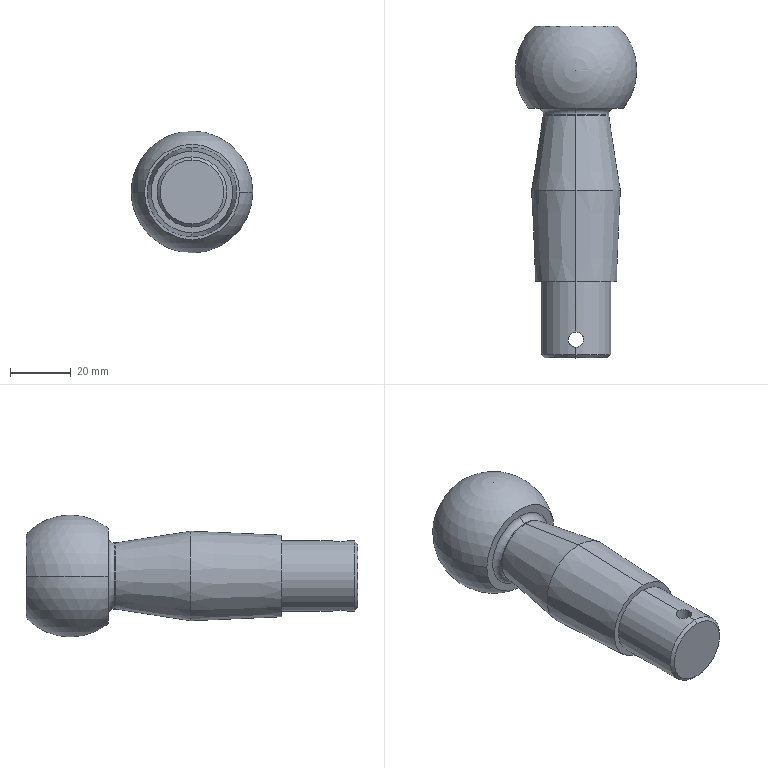Part | SolidWorks | features Chamfer 1, Fillet 1, ICE 1, Revolution 1 | 1 solid | 20 faces | box 40 x 109 x 40 mm | volume 70889 mm3 | cone 6 | torus 4 | cylinder 4 | plane 4 | sphere 2 | commonest cylinder face diameters 5 x2 23 x2
STEP:
#1=CARTESIAN_POINT('',(0.,-12.5,12.835));
#2=VERTEX_POINT('',#1);
#3=CARTESIAN_POINT('',(0.,-14.5,10.835));
#4=VERTEX_POINT('',#3);
#5=CARTESIAN_POINT('',(0.,-14.5,12.835));
#6=DIRECTION('',(-1.,0.,0.));
#7=DIRECTION('',(0.,0.,1.));
#8=AXIS2_PLACEMENT_3D('',#5,#6,#7);
#9=CIRCLE('',#8,2.);
#10=EDGE_CURVE('',#2,#4,#9,.T.);
#11=ORIENTED_EDGE('',*,*,#10,.T.);
#12=CARTESIAN_POINT('',(0.,-14.5,-10.835));
#13=VERTEX_POINT('',#12);
#14=CARTESIAN_POINT('',(0.,-14.5,0.));
#15=DIRECTION('',(0.,1.,0.));
#16=DIRECTION('',(0.,0.,1.));
#17=AXIS2_PLACEMENT_3D('',#14,#15,#16);
#18=CIRCLE('',#17,10.835);
#19=EDGE_CURVE('',#4,#13,#18,.T.);
#20=ORIENTED_EDGE('',*,*,#19,.T.);
#21=CARTESIAN_POINT('',(0.,-12.5,-12.835));
#22=VERTEX_POINT('',#21);
#23=CARTESIAN_POINT('',(0.,-14.5,-12.835));
#24=DIRECTION('',(1.,0.,0.));
#25=DIRECTION('',(0.,0.,-1.));
#26=AXIS2_PLACEMENT_3D('',#23,#24,#25);
#27=CIRCLE('',#26,2.);
#28=EDGE_CURVE('',#22,#13,#27,.T.);
#29=ORIENTED_EDGE('',*,*,#28,.F.);
#30=CARTESIAN_POINT('',(0.,-12.5,0.));
#31=DIRECTION('',(0.,1.,0.));
#32=DIRECTION('',(0.,0.,1.));
#33=AXIS2_PLACEMENT_3D('',#30,#31,#32);
#34=CIRCLE('',#33,12.835);
#35=EDGE_CURVE('',#2,#22,#34,.T.);
#36=ORIENTED_EDGE('',*,*,#35,.F.);
#37=EDGE_LOOP('',(#11,#20,#29,#36));
#38=FACE_OUTER_BOUND('',#37,.T.);
#39=CARTESIAN_POINT('',(0.,-14.5,0.));
#40=DIRECTION('',(0.,1.,0.));
#41=DIRECTION('',(0.,0.,1.));
#42=AXIS2_PLACEMENT_3D('',#39,#40,#41);
#43=TOROIDAL_SURFACE('',#42,12.835,2.);
#44=ADVANCED_FACE('',(#38),#43,.F.);
#45=ORIENTED_EDGE('',*,*,#28,.T.);
#46=CARTESIAN_POINT('',(0.,-14.5,0.));
#47=DIRECTION('',(0.,1.,0.));
#48=DIRECTION('',(0.,0.,1.));
#49=AXIS2_PLACEMENT_3D('',#46,#47,#48);
#50=CIRCLE('',#49,10.835);
#51=EDGE_CURVE('',#13,#4,#50,.T.);
#52=ORIENTED_EDGE('',*,*,#51,.T.);
#53=ORIENTED_EDGE('',*,*,#10,.F.);
#54=CARTESIAN_POINT('',(0.,-12.5,0.));
#55=DIRECTION('',(0.,1.,0.));
#56=DIRECTION('',(0.,0.,1.));
#57=AXIS2_PLACEMENT_3D('',#54,#55,#56);
#58=CIRCLE('',#57,12.835);
#59=EDGE_CURVE('',#22,#2,#58,.T.);
#60=ORIENTED_EDGE('',*,*,#59,.F.);
#61=EDGE_LOOP('',(#45,#52,#53,#60));
#62=FACE_OUTER_BOUND('',#61,.T.);
#63=CARTESIAN_POINT('',(0.,-14.5,0.));
#64=DIRECTION('',(0.,1.,0.));
#65=DIRECTION('',(0.,0.,1.));
#66=AXIS2_PLACEMENT_3D('',#63,#64,#65);
#67=TOROIDAL_SURFACE('',#66,12.835,2.);
#68=ADVANCED_FACE('',(#62),#67,.F.);
#69=CARTESIAN_POINT('',(-2.5,-88.5,-11.225));
#70=VERTEX_POINT('',#69);
#71=CARTESIAN_POINT('',(0.,-91.,-11.5));
#72=VERTEX_POINT('',#71);
#73=CARTESIAN_POINT('',(-2.5,-88.5,-11.225));
#74=CARTESIAN_POINT('',(-2.5,-88.827,-11.225));
#75=CARTESIAN_POINT('',(-2.434,-89.157,-11.24));
#76=CARTESIAN_POINT('',(-2.247,-89.608,-11.279));
#77=CARTESIAN_POINT('',(-2.169,-89.754,-11.294));
#78=CARTESIAN_POINT('',(-1.987,-90.026,-11.327));
#79=CARTESIAN_POINT('',(-1.884,-90.152,-11.345));
#80=CARTESIAN_POINT('',(-1.653,-90.382,-11.381));
#81=CARTESIAN_POINT('',(-1.525,-90.488,-11.399));
#82=CARTESIAN_POINT('',(-1.254,-90.669,-11.432));
#83=CARTESIAN_POINT('',(-1.111,-90.746,-11.447));
#84=CARTESIAN_POINT('',(-0.6555,-90.935,-11.485));
#85=CARTESIAN_POINT('',(-0.3301,-91.,-11.5));
#86=CARTESIAN_POINT('',(0.,-91.,-11.5));
#87=B_SPLINE_CURVE_WITH_KNOTS('',3,(#73,#74,#75,#76,#77,#78,#79,#80,#81,#82,#83,#84,#85,#86),.UNSPECIFIED.,.F.,.F.,(4,2,2,2,2,2,4),(0.00784,0.00882,0.009309,0.009799,0.01029,0.01078,0.01176),.UNSPECIFIED.);
#88=EDGE_CURVE('',#70,#72,#87,.T.);
#89=ORIENTED_EDGE('',*,*,#88,.F.);
#90=CARTESIAN_POINT('',(-2.5,-88.5,11.225));
#91=VERTEX_POINT('',#90);
#92=CARTESIAN_POINT('',(-2.5,-88.5,-20.));
#93=DIRECTION('',(0.,0.,1.));
#94=VECTOR('',#93,1000.);
#95=LINE('',#92,#94);
#96=EDGE_CURVE('',#70,#91,#95,.T.);
#97=ORIENTED_EDGE('',*,*,#96,.T.);
#98=CARTESIAN_POINT('',(0.,-91.,11.5));
#99=VERTEX_POINT('',#98);
#100=CARTESIAN_POINT('',(0.,-91.,11.5));
#101=CARTESIAN_POINT('',(-0.1658,-91.,11.5));
#102=CARTESIAN_POINT('',(-0.3286,-90.984,11.496));
#103=CARTESIAN_POINT('',(-0.6489,-90.92,11.483));
#104=CARTESIAN_POINT('',(-0.8081,-90.871,11.473));
#105=CARTESIAN_POINT('',(-1.111,-90.746,11.447));
#106=CARTESIAN_POINT('',(-1.254,-90.669,11.432));
#107=CARTESIAN_POINT('',(-1.526,-90.487,11.399));
#108=CARTESIAN_POINT('',(-1.654,-90.382,11.381));
#109=CARTESIAN_POINT('',(-1.998,-90.037,11.327));
#110=CARTESIAN_POINT('',(-2.184,-89.759,11.291));
#111=CARTESIAN_POINT('',(-2.372,-89.307,11.253));
#112=CARTESIAN_POINT('',(-2.42,-89.149,11.243));
#113=CARTESIAN_POINT('',(-2.484,-88.826,11.229));
#114=CARTESIAN_POINT('',(-2.5,-88.664,11.225));
#115=CARTESIAN_POINT('',(-2.5,-88.5,11.225));
#116=B_SPLINE_CURVE_WITH_KNOTS('',3,(#100,#101,#102,#103,#104,#105,#106,#107,#108,#109,#110,#111,#112,#113,#114,#115),.UNSPECIFIED.,.F.,.F.,(4,2,2,2,2,2,2,4),(0.,0.0004901,0.0009802,0.00147,0.00196,0.002941,0.003431,0.003921),.UNSPECIFIED.);
#117=EDGE_CURVE('',#99,#91,#116,.T.);
#118=ORIENTED_EDGE('',*,*,#117,.F.);
#119=CARTESIAN_POINT('',(2.5,-88.5,11.225));
#120=VERTEX_POINT('',#119);
#121=CARTESIAN_POINT('',(2.5,-88.5,11.225));
#122=CARTESIAN_POINT('',(2.5,-88.665,11.225));
#123=CARTESIAN_POINT('',(2.484,-88.828,11.229));
#124=CARTESIAN_POINT('',(2.42,-89.148,11.243));
#125=CARTESIAN_POINT('',(2.372,-89.307,11.253));
#126=CARTESIAN_POINT('',(2.246,-89.609,11.279));
#127=CARTESIAN_POINT('',(2.17,-89.753,11.294));
#128=CARTESIAN_POINT('',(1.988,-90.025,11.327));
#129=CARTESIAN_POINT('',(1.883,-90.152,11.345));
#130=CARTESIAN_POINT('',(1.539,-90.497,11.399));
#131=CARTESIAN_POINT('',(1.261,-90.683,11.435));
#132=CARTESIAN_POINT('',(0.8102,-90.871,11.472));
#133=CARTESIAN_POINT('',(0.6514,-90.919,11.483));
#134=CARTESIAN_POINT('',(0.329,-90.984,11.496));
#135=CARTESIAN_POINT('',(0.1656,-91.,11.5));
#136=CARTESIAN_POINT('',(0.,-91.,11.5));
#137=B_SPLINE_CURVE_WITH_KNOTS('',3,(#121,#122,#123,#124,#125,#126,#127,#128,#129,#130,#131,#132,#133,#134,#135,#136),.UNSPECIFIED.,.F.,.F.,(4,2,2,2,2,2,2,4),(0.01176,0.01225,0.01274,0.01323,0.01372,0.0147,0.01519,0.01568),.UNSPECIFIED.);
#138=EDGE_CURVE('',#120,#99,#137,.T.);
#139=ORIENTED_EDGE('',*,*,#138,.F.);
#140=CARTESIAN_POINT('',(2.5,-88.5,-11.225));
#141=VERTEX_POINT('',#140);
#142=CARTESIAN_POINT('',(2.5,-88.5,-20.));
#143=DIRECTION('',(0.,0.,1.));
#144=VECTOR('',#143,1000.);
#145=LINE('',#142,#144);
#146=EDGE_CURVE('',#141,#120,#145,.T.);
#147=ORIENTED_EDGE('',*,*,#146,.F.);
#148=CARTESIAN_POINT('',(0.,-91.,-11.5));
#149=CARTESIAN_POINT('',(0.1649,-91.,-11.5));
#150=CARTESIAN_POINT('',(0.3275,-90.984,-11.496));
#151=CARTESIAN_POINT('',(0.648,-90.92,-11.483));
#152=CARTESIAN_POINT('',(0.8074,-90.872,-11.473));
#153=CARTESIAN_POINT('',(1.109,-90.746,-11.447));
#154=CARTESIAN_POINT('',(1.253,-90.67,-11.432));
#155=CARTESIAN_POINT('',(1.525,-90.488,-11.399));
#156=CARTESIAN_POINT('',(1.652,-90.383,-11.381));
#157=CARTESIAN_POINT('',(1.997,-90.039,-11.328));
#158=CARTESIAN_POINT('',(2.183,-89.761,-11.292));
#159=CARTESIAN_POINT('',(2.371,-89.31,-11.253));
#160=CARTESIAN_POINT('',(2.419,-89.151,-11.243));
#161=CARTESIAN_POINT('',(2.484,-88.829,-11.229));
#162=CARTESIAN_POINT('',(2.5,-88.666,-11.225));
#163=CARTESIAN_POINT('',(2.5,-88.5,-11.225));
#164=B_SPLINE_CURVE_WITH_KNOTS('',3,(#148,#149,#150,#151,#152,#153,#154,#155,#156,#157,#158,#159,#160,#161,#162,#163),.UNSPECIFIED.,.F.,.F.,(4,2,2,2,2,2,2,4),(0.01176,0.01225,0.01274,0.01323,0.01372,0.0147,0.01519,0.01568),.UNSPECIFIED.);
#165=EDGE_CURVE('',#72,#141,#164,.T.);
#166=ORIENTED_EDGE('',*,*,#165,.F.);
#167=EDGE_LOOP('',(#89,#97,#118,#139,#147,#166));
#168=FACE_OUTER_BOUND('',#167,.T.);
#169=CARTESIAN_POINT('',(0.,-88.5,-20.));
#170=DIRECTION('',(0.,0.,1.));
#171=DIRECTION('',(1.,0.,0.));
#172=AXIS2_PLACEMENT_3D('',#169,#170,#171);
#173=CYLINDRICAL_SURFACE('',#172,2.5);
#174=ADVANCED_FACE('',(#168),#173,.F.);
#175=ORIENTED_EDGE('',*,*,#51,.F.);
#176=CARTESIAN_POINT('',(0.,-14.807,-10.859));
#177=VERTEX_POINT('',#176);
#178=CARTESIAN_POINT('',(0.,-14.5,-12.835));
#179=DIRECTION('',(1.,0.,0.));
#180=DIRECTION('',(0.,0.,-1.));
#181=AXIS2_PLACEMENT_3D('',#178,#179,#180);
#182=CIRCLE('',#181,2.);
#183=EDGE_CURVE('',#13,#177,#182,.T.);
#184=ORIENTED_EDGE('',*,*,#183,.T.);
#185=CARTESIAN_POINT('',(0.,-14.807,10.859));
#186=VERTEX_POINT('',#185);
#187=CARTESIAN_POINT('',(0.,-14.807,0.));
#188=DIRECTION('',(0.,-1.,0.));
#189=DIRECTION('',(0.,0.,-1.));
#190=AXIS2_PLACEMENT_3D('',#187,#188,#189);
#191=CIRCLE('',#190,10.859);
#192=EDGE_CURVE('',#186,#177,#191,.T.);
#193=ORIENTED_EDGE('',*,*,#192,.F.);
#194=CARTESIAN_POINT('',(0.,-14.5,12.835));
#195=DIRECTION('',(-1.,0.,0.));
#196=DIRECTION('',(0.,0.,1.));
#197=AXIS2_PLACEMENT_3D('',#194,#195,#196);
#198=CIRCLE('',#197,2.);
#199=EDGE_CURVE('',#4,#186,#198,.T.);
#200=ORIENTED_EDGE('',*,*,#199,.F.);
#201=EDGE_LOOP('',(#175,#184,#193,#200));
#202=FACE_OUTER_BOUND('',#201,.T.);
#203=CARTESIAN_POINT('',(0.,-14.5,0.));
#204=DIRECTION('',(0.,1.,0.));
#205=DIRECTION('',(0.,0.,1.));
#206=AXIS2_PLACEMENT_3D('',#203,#204,#205);
#207=TOROIDAL_SURFACE('',#206,12.835,2.);
#208=ADVANCED_FACE('',(#202),#207,.F.);
#209=CARTESIAN_POINT('',(0.,-94.5,-10.5));
#210=VERTEX_POINT('',#209);
#211=CARTESIAN_POINT('',(0.,-94.5,10.5));
#212=VERTEX_POINT('',#211);
#213=CARTESIAN_POINT('',(0.,-94.5,0.));
#214=DIRECTION('',(0.,-1.,0.));
#215=DIRECTION('',(0.,0.,1.));
#216=AXIS2_PLACEMENT_3D('',#213,#214,#215);
#217=CIRCLE('',#216,10.5);
#218=EDGE_CURVE('',#210,#212,#217,.T.);
#219=ORIENTED_EDGE('',*,*,#218,.F.);
#220=CARTESIAN_POINT('',(0.,-93.5,-11.5));
#221=VERTEX_POINT('',#220);
#222=CARTESIAN_POINT('',(0.,-93.5,-11.5));
#223=DIRECTION('',(0.,0.7071,-0.7071));
#224=VECTOR('',#223,1000.);
#225=LINE('',#222,#224);
#226=EDGE_CURVE('',#210,#221,#225,.T.);
#227=ORIENTED_EDGE('',*,*,#226,.T.);
#228=CARTESIAN_POINT('',(0.,-93.5,11.5));
#229=VERTEX_POINT('',#228);
#230=CARTESIAN_POINT('',(0.,-93.5,0.));
#231=DIRECTION('',(0.,1.,0.));
#232=DIRECTION('',(0.,0.,1.));
#233=AXIS2_PLACEMENT_3D('',#230,#231,#232);
#234=CIRCLE('',#233,11.5);
#235=EDGE_CURVE('',#229,#221,#234,.T.);
#236=ORIENTED_EDGE('',*,*,#235,.F.);
#237=CARTESIAN_POINT('',(0.,-93.5,11.5));
#238=DIRECTION('',(0.,0.7071,0.7071));
#239=VECTOR('',#238,1000.);
#240=LINE('',#237,#239);
#241=EDGE_CURVE('',#212,#229,#240,.T.);
#242=ORIENTED_EDGE('',*,*,#241,.F.);
#243=EDGE_LOOP('',(#219,#227,#236,#242));
#244=FACE_OUTER_BOUND('',#243,.T.);
#245=CARTESIAN_POINT('',(0.,-93.5,0.));
#246=DIRECTION('',(0.,1.,0.));
#247=DIRECTION('',(0.,0.,1.));
#248=AXIS2_PLACEMENT_3D('',#245,#246,#247);
#249=CONICAL_SURFACE('',#248,11.5,0.7854);
#250=ADVANCED_FACE('',(#244),#249,.T.);
#251=CARTESIAN_POINT('',(15.612,-12.5,0.));
#252=VERTEX_POINT('',#251);
#253=CARTESIAN_POINT('',(-15.612,-12.5,0.));
#254=VERTEX_POINT('',#253);
#255=CARTESIAN_POINT('',(0.,-12.5,0.));
#256=DIRECTION('',(0.,1.,0.));
#257=DIRECTION('',(0.,0.,1.));
#258=AXIS2_PLACEMENT_3D('',#255,#256,#257);
#259=CIRCLE('',#258,15.612);
#260=EDGE_CURVE('',#252,#254,#259,.T.);
#261=ORIENTED_EDGE('',*,*,#260,.T.);
#262=CARTESIAN_POINT('',(-13.775,14.5,0.));
#263=VERTEX_POINT('',#262);
#264=CARTESIAN_POINT('',(0.,0.,0.));
#265=DIRECTION('',(0.,0.,-1.));
#266=DIRECTION('',(-1.,0.,0.));
#267=AXIS2_PLACEMENT_3D('',#264,#265,#266);
#268=CIRCLE('',#267,20.);
#269=EDGE_CURVE('',#254,#263,#268,.T.);
#270=ORIENTED_EDGE('',*,*,#269,.T.);
#271=CARTESIAN_POINT('',(13.775,14.5,0.));
#272=VERTEX_POINT('',#271);
#273=CARTESIAN_POINT('',(0.,14.5,0.));
#274=DIRECTION('',(0.,1.,0.));
#275=DIRECTION('',(0.,0.,1.));
#276=AXIS2_PLACEMENT_3D('',#273,#274,#275);
#277=CIRCLE('',#276,13.775);
#278=EDGE_CURVE('',#272,#263,#277,.T.);
#279=ORIENTED_EDGE('',*,*,#278,.F.);
#280=CARTESIAN_POINT('',(0.,0.,0.));
#281=DIRECTION('',(0.,0.,1.));
#282=DIRECTION('',(1.,0.,0.));
#283=AXIS2_PLACEMENT_3D('',#280,#281,#282);
#284=CIRCLE('',#283,20.);
#285=EDGE_CURVE('',#252,#272,#284,.T.);
#286=ORIENTED_EDGE('',*,*,#285,.F.);
#287=EDGE_LOOP('',(#261,#270,#279,#286));
#288=FACE_OUTER_BOUND('',#287,.T.);
#289=CARTESIAN_POINT('',(0.,0.,0.));
#290=DIRECTION('',(0.,0.,-1.));
#291=DIRECTION('',(1.,0.,0.));
#292=AXIS2_PLACEMENT_3D('',#289,#290,#291);
#293=SPHERICAL_SURFACE('',#292,20.);
#294=ADVANCED_FACE('',(#288),#293,.T.);
#295=CARTESIAN_POINT('',(0.,-14.807,0.));
#296=DIRECTION('',(0.,-1.,0.));
#297=DIRECTION('',(0.,0.,-1.));
#298=AXIS2_PLACEMENT_3D('',#295,#296,#297);
#299=CIRCLE('',#298,10.859);
#300=EDGE_CURVE('',#177,#186,#299,.T.);
#301=ORIENTED_EDGE('',*,*,#300,.T.);
#302=CARTESIAN_POINT('',(0.,-39.5,14.7));
#303=VERTEX_POINT('',#302);
#304=CARTESIAN_POINT('',(0.,-39.5,14.7));
#305=DIRECTION('',(0.,-0.9881,0.1537));
#306=VECTOR('',#305,1000.);
#307=LINE('',#304,#306);
#308=EDGE_CURVE('',#186,#303,#307,.T.);
#309=ORIENTED_EDGE('',*,*,#308,.T.);
#310=CARTESIAN_POINT('',(0.,-39.5,-14.7));
#311=VERTEX_POINT('',#310);
#312=CARTESIAN_POINT('',(0.,-39.5,0.));
#313=DIRECTION('',(0.,1.,0.));
#314=DIRECTION('',(0.,0.,1.));
#315=AXIS2_PLACEMENT_3D('',#312,#313,#314);
#316=CIRCLE('',#315,14.7);
#317=EDGE_CURVE('',#303,#311,#316,.T.);
#318=ORIENTED_EDGE('',*,*,#317,.T.);
#319=CARTESIAN_POINT('',(0.,-39.5,-14.7));
#320=DIRECTION('',(0.,-0.9881,-0.1537));
#321=VECTOR('',#320,1000.);
#322=LINE('',#319,#321);
#323=EDGE_CURVE('',#177,#311,#322,.T.);
#324=ORIENTED_EDGE('',*,*,#323,.F.);
#325=EDGE_LOOP('',(#301,#309,#318,#324));
#326=FACE_OUTER_BOUND('',#325,.T.);
#327=CARTESIAN_POINT('',(0.,-39.5,0.));
#328=DIRECTION('',(0.,-1.,0.));
#329=DIRECTION('',(0.,0.,-1.));
#330=AXIS2_PLACEMENT_3D('',#327,#328,#329);
#331=CONICAL_SURFACE('',#330,14.7,0.1543);
#332=ADVANCED_FACE('',(#326),#331,.T.);
#333=CARTESIAN_POINT('',(0.,-69.5,13.4));
#334=VERTEX_POINT('',#333);
#335=CARTESIAN_POINT('',(0.,-69.5,-13.4));
#336=VERTEX_POINT('',#335);
#337=CARTESIAN_POINT('',(0.,-69.5,0.));
#338=DIRECTION('',(0.,1.,0.));
#339=DIRECTION('',(0.,0.,1.));
#340=AXIS2_PLACEMENT_3D('',#337,#338,#339);
#341=CIRCLE('',#340,13.4);
#342=EDGE_CURVE('',#334,#336,#341,.T.);
#343=ORIENTED_EDGE('',*,*,#342,.T.);
#344=CARTESIAN_POINT('',(0.,-69.5,-13.4));
#345=DIRECTION('',(0.,0.9991,-0.04329));
#346=VECTOR('',#345,1000.);
#347=LINE('',#344,#346);
#348=EDGE_CURVE('',#336,#311,#347,.T.);
#349=ORIENTED_EDGE('',*,*,#348,.T.);
#350=ORIENTED_EDGE('',*,*,#317,.F.);
#351=CARTESIAN_POINT('',(0.,-69.5,13.4));
#352=DIRECTION('',(0.,0.9991,0.04329));
#353=VECTOR('',#352,1000.);
#354=LINE('',#351,#353);
#355=EDGE_CURVE('',#334,#303,#354,.T.);
#356=ORIENTED_EDGE('',*,*,#355,.F.);
#357=EDGE_LOOP('',(#343,#349,#350,#356));
#358=FACE_OUTER_BOUND('',#357,.T.);
#359=CARTESIAN_POINT('',(0.,-69.5,0.));
#360=DIRECTION('',(0.,1.,0.));
#361=DIRECTION('',(0.,0.,1.));
#362=AXIS2_PLACEMENT_3D('',#359,#360,#361);
#363=CONICAL_SURFACE('',#362,13.4,0.04331);
#364=ADVANCED_FACE('',(#358),#363,.T.);
#365=ORIENTED_EDGE('',*,*,#235,.T.);
#366=CARTESIAN_POINT('',(0.,41.044,-11.5));
#367=DIRECTION('',(0.,1.,0.));
#368=VECTOR('',#367,1000.);
#369=LINE('',#366,#368);
#370=EDGE_CURVE('',#221,#72,#369,.T.);
#371=ORIENTED_EDGE('',*,*,#370,.T.);
#372=ORIENTED_EDGE('',*,*,#165,.T.);
#373=CARTESIAN_POINT('',(0.,-86.,-11.5));
#374=VERTEX_POINT('',#373);
#375=CARTESIAN_POINT('',(2.5,-88.5,-11.225));
#376=CARTESIAN_POINT('',(2.5,-88.334,-11.225));
#377=CARTESIAN_POINT('',(2.484,-88.171,-11.229));
#378=CARTESIAN_POINT('',(2.42,-87.851,-11.243));
#379=CARTESIAN_POINT('',(2.371,-87.692,-11.253));
#380=CARTESIAN_POINT('',(2.246,-87.389,-11.279));
#381=CARTESIAN_POINT('',(2.169,-87.246,-11.294));
#382=CARTESIAN_POINT('',(1.987,-86.975,-11.327));
#383=CARTESIAN_POINT('',(1.882,-86.846,-11.346));
#384=CARTESIAN_POINT('',(1.537,-86.502,-11.399));
#385=CARTESIAN_POINT('',(1.259,-86.316,-11.435));
#386=CARTESIAN_POINT('',(0.8075,-86.128,-11.473));
#387=CARTESIAN_POINT('',(0.6493,-86.08,-11.483));
#388=CARTESIAN_POINT('',(0.3263,-86.016,-11.497));
#389=CARTESIAN_POINT('',(0.1637,-86.,-11.5));
#390=CARTESIAN_POINT('',(0.,-86.,-11.5));
#391=B_SPLINE_CURVE_WITH_KNOTS('',3,(#375,#376,#377,#378,#379,#380,#381,#382,#383,#384,#385,#386,#387,#388,#389,#390),.UNSPECIFIED.,.F.,.F.,(4,2,2,2,2,2,2,4),(0.,0.0004901,0.0009802,0.00147,0.00196,0.002941,0.003431,0.003921),.UNSPECIFIED.);
#392=EDGE_CURVE('',#141,#374,#391,.T.);
#393=ORIENTED_EDGE('',*,*,#392,.T.);
#394=CARTESIAN_POINT('',(0.,-69.5,-11.5));
#395=VERTEX_POINT('',#394);
#396=CARTESIAN_POINT('',(0.,41.044,-11.5));
#397=DIRECTION('',(0.,1.,0.));
#398=VECTOR('',#397,1000.);
#399=LINE('',#396,#398);
#400=EDGE_CURVE('',#374,#395,#399,.T.);
#401=ORIENTED_EDGE('',*,*,#400,.T.);
#402=CARTESIAN_POINT('',(0.,-69.5,11.5));
#403=VERTEX_POINT('',#402);
#404=CARTESIAN_POINT('',(0.,-69.5,0.));
#405=DIRECTION('',(0.,1.,0.));
#406=DIRECTION('',(0.,0.,1.));
#407=AXIS2_PLACEMENT_3D('',#404,#405,#406);
#408=CIRCLE('',#407,11.5);
#409=EDGE_CURVE('',#403,#395,#408,.T.);
#410=ORIENTED_EDGE('',*,*,#409,.F.);
#411=CARTESIAN_POINT('',(0.,-86.,11.5));
#412=VERTEX_POINT('',#411);
#413=CARTESIAN_POINT('',(0.,41.044,11.5));
#414=DIRECTION('',(0.,1.,0.));
#415=VECTOR('',#414,1000.);
#416=LINE('',#413,#415);
#417=EDGE_CURVE('',#412,#403,#416,.T.);
#418=ORIENTED_EDGE('',*,*,#417,.F.);
#419=CARTESIAN_POINT('',(0.,-86.,11.5));
#420=CARTESIAN_POINT('',(0.3269,-86.,11.5));
#421=CARTESIAN_POINT('',(0.6568,-86.066,11.485));
#422=CARTESIAN_POINT('',(1.108,-86.253,11.447));
#423=CARTESIAN_POINT('',(1.255,-86.331,11.432));
#424=CARTESIAN_POINT('',(1.526,-86.513,11.399));
#425=CARTESIAN_POINT('',(1.652,-86.616,11.381));
#426=CARTESIAN_POINT('',(1.883,-86.847,11.345));
#427=CARTESIAN_POINT('',(1.988,-86.975,11.327));
#428=CARTESIAN_POINT('',(2.169,-87.246,11.294));
#429=CARTESIAN_POINT('',(2.246,-87.389,11.279));
#430=CARTESIAN_POINT('',(2.435,-87.845,11.24));
#431=CARTESIAN_POINT('',(2.5,-88.17,11.225));
#432=CARTESIAN_POINT('',(2.5,-88.5,11.225));
#433=B_SPLINE_CURVE_WITH_KNOTS('',3,(#419,#420,#421,#422,#423,#424,#425,#426,#427,#428,#429,#430,#431,#432),.UNSPECIFIED.,.F.,.F.,(4,2,2,2,2,2,4),(0.00784,0.00882,0.00931,0.0098,0.01029,0.01078,0.01176),.UNSPECIFIED.);
#434=EDGE_CURVE('',#412,#120,#433,.T.);
#435=ORIENTED_EDGE('',*,*,#434,.T.);
#436=ORIENTED_EDGE('',*,*,#138,.T.);
#437=CARTESIAN_POINT('',(0.,41.044,11.5));
#438=DIRECTION('',(0.,1.,0.));
#439=VECTOR('',#438,1000.);
#440=LINE('',#437,#439);
#441=EDGE_CURVE('',#229,#99,#440,.T.);
#442=ORIENTED_EDGE('',*,*,#441,.F.);
#443=EDGE_LOOP('',(#365,#371,#372,#393,#401,#410,#418,#435,#436,#442));
#444=FACE_OUTER_BOUND('',#443,.T.);
#445=CARTESIAN_POINT('',(0.,41.044,0.));
#446=DIRECTION('',(0.,1.,0.));
#447=DIRECTION('',(0.,0.,1.));
#448=AXIS2_PLACEMENT_3D('',#445,#446,#447);
#449=CYLINDRICAL_SURFACE('',#448,11.5);
#450=ADVANCED_FACE('',(#444),#449,.T.);
#451=ORIENTED_EDGE('',*,*,#278,.T.);
#452=CARTESIAN_POINT('',(0.,14.5,0.));
#453=DIRECTION('',(0.,1.,0.));
#454=DIRECTION('',(0.,0.,1.));
#455=AXIS2_PLACEMENT_3D('',#452,#453,#454);
#456=CIRCLE('',#455,13.775);
#457=EDGE_CURVE('',#263,#272,#456,.T.);
#458=ORIENTED_EDGE('',*,*,#457,.T.);
#459=EDGE_LOOP('',(#451,#458));
#460=FACE_OUTER_BOUND('',#459,.T.);
#461=CARTESIAN_POINT('',(0.,14.5,0.));
#462=DIRECTION('',(0.,-1.,0.));
#463=DIRECTION('',(0.,0.,-1.));
#464=AXIS2_PLACEMENT_3D('',#461,#462,#463);
#465=PLANE('',#464);
#466=ADVANCED_FACE('',(#460),#465,.F.);
#467=CARTESIAN_POINT('',(0.,-94.5,0.));
#468=DIRECTION('',(0.,-1.,0.));
#469=DIRECTION('',(0.,0.,1.));
#470=AXIS2_PLACEMENT_3D('',#467,#468,#469);
#471=CIRCLE('',#470,10.5);
#472=EDGE_CURVE('',#212,#210,#471,.T.);
#473=ORIENTED_EDGE('',*,*,#472,.T.);
#474=ORIENTED_EDGE('',*,*,#218,.T.);
#475=EDGE_LOOP('',(#473,#474));
#476=FACE_OUTER_BOUND('',#475,.T.);
#477=CARTESIAN_POINT('',(11.5,-94.5,0.));
#478=DIRECTION('',(0.,1.,0.));
#479=DIRECTION('',(0.,0.,1.));
#480=AXIS2_PLACEMENT_3D('',#477,#478,#479);
#481=PLANE('',#480);
#482=ADVANCED_FACE('',(#476),#481,.F.);
#483=ORIENTED_EDGE('',*,*,#370,.F.);
#484=CARTESIAN_POINT('',(0.,-93.5,0.));
#485=DIRECTION('',(0.,1.,0.));
#486=DIRECTION('',(0.,0.,1.));
#487=AXIS2_PLACEMENT_3D('',#484,#485,#486);
#488=CIRCLE('',#487,11.5);
#489=EDGE_CURVE('',#221,#229,#488,.T.);
#490=ORIENTED_EDGE('',*,*,#489,.T.);
#491=ORIENTED_EDGE('',*,*,#441,.T.);
#492=ORIENTED_EDGE('',*,*,#117,.T.);
#493=CARTESIAN_POINT('',(-2.5,-88.5,11.225));
#494=CARTESIAN_POINT('',(-2.5,-88.336,11.225));
#495=CARTESIAN_POINT('',(-2.484,-88.17,11.229));
#496=CARTESIAN_POINT('',(-2.419,-87.849,11.243));
#497=CARTESIAN_POINT('',(-2.372,-87.693,11.253));
#498=CARTESIAN_POINT('',(-2.246,-87.39,11.279));
#499=CARTESIAN_POINT('',(-2.168,-87.245,11.294));
#500=CARTESIAN_POINT('',(-1.987,-86.974,11.327));
#501=CARTESIAN_POINT('',(-1.883,-86.848,11.345));
#502=CARTESIAN_POINT('',(-1.651,-86.616,11.381));
#503=CARTESIAN_POINT('',(-1.525,-86.513,11.399));
#504=CARTESIAN_POINT('',(-1.255,-86.332,11.432));
#505=CARTESIAN_POINT('',(-1.109,-86.253,11.447));
#506=CARTESIAN_POINT('',(-0.8066,-86.128,11.473));
#507=CARTESIAN_POINT('',(-0.6508,-86.081,11.483));
#508=CARTESIAN_POINT('',(-0.3293,-86.016,11.496));
#509=CARTESIAN_POINT('',(-0.1634,-86.,11.5));
#510=CARTESIAN_POINT('',(0.,-86.,11.5));
#511=B_SPLINE_CURVE_WITH_KNOTS('',3,(#493,#494,#495,#496,#497,#498,#499,#500,#501,#502,#503,#504,#505,#506,#507,#508,#509,#510),.UNSPECIFIED.,.F.,.F.,(4,2,2,2,2,2,2,2,4),(0.003921,0.004411,0.0049,0.00539,0.00588,0.00637,0.00686,0.00735,0.00784),.UNSPECIFIED.);
#512=EDGE_CURVE('',#91,#412,#511,.T.);
#513=ORIENTED_EDGE('',*,*,#512,.T.);
#514=ORIENTED_EDGE('',*,*,#417,.T.);
#515=CARTESIAN_POINT('',(0.,-69.5,0.));
#516=DIRECTION('',(0.,1.,0.));
#517=DIRECTION('',(0.,0.,1.));
#518=AXIS2_PLACEMENT_3D('',#515,#516,#517);
#519=CIRCLE('',#518,11.5);
#520=EDGE_CURVE('',#395,#403,#519,.T.);
#521=ORIENTED_EDGE('',*,*,#520,.F.);
#522=ORIENTED_EDGE('',*,*,#400,.F.);
#523=CARTESIAN_POINT('',(0.,-86.,-11.5));
#524=CARTESIAN_POINT('',(-0.1636,-86.,-11.5));
#525=CARTESIAN_POINT('',(-0.3298,-86.016,-11.496));
#526=CARTESIAN_POINT('',(-0.6507,-86.081,-11.483));
#527=CARTESIAN_POINT('',(-0.8067,-86.128,-11.473));
#528=CARTESIAN_POINT('',(-1.11,-86.254,-11.447));
#529=CARTESIAN_POINT('',(-1.255,-86.332,-11.432));
#530=CARTESIAN_POINT('',(-1.526,-86.513,-11.399));
#531=CARTESIAN_POINT('',(-1.652,-86.617,-11.381));
#532=CARTESIAN_POINT('',(-1.884,-86.849,-11.345));
#533=CARTESIAN_POINT('',(-1.987,-86.975,-11.327));
#534=CARTESIAN_POINT('',(-2.168,-87.245,-11.294));
#535=CARTESIAN_POINT('',(-2.247,-87.391,-11.279));
#536=CARTESIAN_POINT('',(-2.372,-87.693,-11.253));
#537=CARTESIAN_POINT('',(-2.419,-87.849,-11.243));
#538=CARTESIAN_POINT('',(-2.484,-88.171,-11.229));
#539=CARTESIAN_POINT('',(-2.5,-88.337,-11.225));
#540=CARTESIAN_POINT('',(-2.5,-88.5,-11.225));
#541=B_SPLINE_CURVE_WITH_KNOTS('',3,(#523,#524,#525,#526,#527,#528,#529,#530,#531,#532,#533,#534,#535,#536,#537,#538,#539,#540),.UNSPECIFIED.,.F.,.F.,(4,2,2,2,2,2,2,2,4),(0.003921,0.004411,0.0049,0.00539,0.00588,0.00637,0.00686,0.00735,0.00784),.UNSPECIFIED.);
#542=EDGE_CURVE('',#374,#70,#541,.T.);
#543=ORIENTED_EDGE('',*,*,#542,.T.);
#544=ORIENTED_EDGE('',*,*,#88,.T.);
#545=EDGE_LOOP('',(#483,#490,#491,#492,#513,#514,#521,#522,#543,#544));
#546=FACE_OUTER_BOUND('',#545,.T.);
#547=CARTESIAN_POINT('',(0.,41.044,0.));
#548=DIRECTION('',(0.,1.,0.));
#549=DIRECTION('',(0.,0.,1.));
#550=AXIS2_PLACEMENT_3D('',#547,#548,#549);
#551=CYLINDRICAL_SURFACE('',#550,11.5);
#552=ADVANCED_FACE('',(#546),#551,.T.);
#553=ORIENTED_EDGE('',*,*,#342,.F.);
#554=CARTESIAN_POINT('',(0.,-69.5,0.));
#555=DIRECTION('',(0.,1.,0.));
#556=DIRECTION('',(0.,0.,1.));
#557=AXIS2_PLACEMENT_3D('',#554,#555,#556);
#558=CIRCLE('',#557,13.4);
#559=EDGE_CURVE('',#336,#334,#558,.T.);
#560=ORIENTED_EDGE('',*,*,#559,.F.);
#561=EDGE_LOOP('',(#553,#560));
#562=FACE_OUTER_BOUND('',#561,.T.);
#563=ORIENTED_EDGE('',*,*,#409,.T.);
#564=ORIENTED_EDGE('',*,*,#520,.T.);
#565=EDGE_LOOP('',(#563,#564));
#566=FACE_BOUND('',#565,.T.);
#567=CARTESIAN_POINT('',(13.4,-69.5,0.));
#568=DIRECTION('',(0.,1.,0.));
#569=DIRECTION('',(0.,0.,1.));
#570=AXIS2_PLACEMENT_3D('',#567,#568,#569);
#571=PLANE('',#570);
#572=ADVANCED_FACE('',(#562,#566),#571,.F.);
#573=ORIENTED_EDGE('',*,*,#348,.F.);
#574=ORIENTED_EDGE('',*,*,#559,.T.);
#575=ORIENTED_EDGE('',*,*,#355,.T.);
#576=CARTESIAN_POINT('',(0.,-39.5,0.));
#577=DIRECTION('',(0.,1.,0.));
#578=DIRECTION('',(0.,0.,1.));
#579=AXIS2_PLACEMENT_3D('',#576,#577,#578);
#580=CIRCLE('',#579,14.7);
#581=EDGE_CURVE('',#311,#303,#580,.T.);
#582=ORIENTED_EDGE('',*,*,#581,.F.);
#583=EDGE_LOOP('',(#573,#574,#575,#582));
#584=FACE_OUTER_BOUND('',#583,.T.);
#585=CARTESIAN_POINT('',(0.,-69.5,0.));
#586=DIRECTION('',(0.,1.,0.));
#587=DIRECTION('',(0.,0.,1.));
#588=AXIS2_PLACEMENT_3D('',#585,#586,#587);
#589=CONICAL_SURFACE('',#588,13.4,0.04331);
#590=ADVANCED_FACE('',(#584),#589,.T.);
#591=ORIENTED_EDGE('',*,*,#308,.F.);
#592=ORIENTED_EDGE('',*,*,#192,.T.);
#593=ORIENTED_EDGE('',*,*,#323,.T.);
#594=ORIENTED_EDGE('',*,*,#581,.T.);
#595=EDGE_LOOP('',(#591,#592,#593,#594));
#596=FACE_OUTER_BOUND('',#595,.T.);
#597=CARTESIAN_POINT('',(0.,-39.5,0.));
#598=DIRECTION('',(0.,-1.,0.));
#599=DIRECTION('',(0.,0.,-1.));
#600=AXIS2_PLACEMENT_3D('',#597,#598,#599);
#601=CONICAL_SURFACE('',#600,14.7,0.1543);
#602=ADVANCED_FACE('',(#596),#601,.T.);
#603=ORIENTED_EDGE('',*,*,#35,.T.);
#604=ORIENTED_EDGE('',*,*,#59,.T.);
#605=EDGE_LOOP('',(#603,#604));
#606=FACE_BOUND('',#605,.T.);
#607=ORIENTED_EDGE('',*,*,#260,.F.);
#608=CARTESIAN_POINT('',(0.,-12.5,0.));
#609=DIRECTION('',(0.,1.,0.));
#610=DIRECTION('',(0.,0.,1.));
#611=AXIS2_PLACEMENT_3D('',#608,#609,#610);
#612=CIRCLE('',#611,15.612);
#613=EDGE_CURVE('',#254,#252,#612,.T.);
#614=ORIENTED_EDGE('',*,*,#613,.F.);
#615=EDGE_LOOP('',(#607,#614));
#616=FACE_OUTER_BOUND('',#615,.T.);
#617=CARTESIAN_POINT('',(10.5,-12.5,0.));
#618=DIRECTION('',(0.,1.,0.));
#619=DIRECTION('',(0.,0.,1.));
#620=AXIS2_PLACEMENT_3D('',#617,#618,#619);
#621=PLANE('',#620);
#622=ADVANCED_FACE('',(#606,#616),#621,.F.);
#623=ORIENTED_EDGE('',*,*,#269,.F.);
#624=ORIENTED_EDGE('',*,*,#613,.T.);
#625=ORIENTED_EDGE('',*,*,#285,.T.);
#626=ORIENTED_EDGE('',*,*,#457,.F.);
#627=EDGE_LOOP('',(#623,#624,#625,#626));
#628=FACE_OUTER_BOUND('',#627,.T.);
#629=CARTESIAN_POINT('',(0.,0.,0.));
#630=DIRECTION('',(0.,0.,-1.));
#631=DIRECTION('',(1.,0.,0.));
#632=AXIS2_PLACEMENT_3D('',#629,#630,#631);
#633=SPHERICAL_SURFACE('',#632,20.);
#634=ADVANCED_FACE('',(#628),#633,.T.);
#635=ORIENTED_EDGE('',*,*,#226,.F.);
#636=ORIENTED_EDGE('',*,*,#472,.F.);
#637=ORIENTED_EDGE('',*,*,#241,.T.);
#638=ORIENTED_EDGE('',*,*,#489,.F.);
#639=EDGE_LOOP('',(#635,#636,#637,#638));
#640=FACE_OUTER_BOUND('',#639,.T.);
#641=CARTESIAN_POINT('',(0.,-93.5,0.));
#642=DIRECTION('',(0.,1.,0.));
#643=DIRECTION('',(0.,0.,1.));
#644=AXIS2_PLACEMENT_3D('',#641,#642,#643);
#645=CONICAL_SURFACE('',#644,11.5,0.7854);
#646=ADVANCED_FACE('',(#640),#645,.T.);
#647=ORIENTED_EDGE('',*,*,#19,.F.);
#648=ORIENTED_EDGE('',*,*,#199,.T.);
#649=ORIENTED_EDGE('',*,*,#300,.F.);
#650=ORIENTED_EDGE('',*,*,#183,.F.);
#651=EDGE_LOOP('',(#647,#648,#649,#650));
#652=FACE_OUTER_BOUND('',#651,.T.);
#653=CARTESIAN_POINT('',(0.,-14.5,0.));
#654=DIRECTION('',(0.,1.,0.));
#655=DIRECTION('',(0.,0.,1.));
#656=AXIS2_PLACEMENT_3D('',#653,#654,#655);
#657=TOROIDAL_SURFACE('',#656,12.835,2.);
#658=ADVANCED_FACE('',(#652),#657,.F.);
#659=ORIENTED_EDGE('',*,*,#96,.F.);
#660=ORIENTED_EDGE('',*,*,#542,.F.);
#661=ORIENTED_EDGE('',*,*,#392,.F.);
#662=ORIENTED_EDGE('',*,*,#146,.T.);
#663=ORIENTED_EDGE('',*,*,#434,.F.);
#664=ORIENTED_EDGE('',*,*,#512,.F.);
#665=EDGE_LOOP('',(#659,#660,#661,#662,#663,#664));
#666=FACE_OUTER_BOUND('',#665,.T.);
#667=CARTESIAN_POINT('',(0.,-88.5,-20.));
#668=DIRECTION('',(0.,0.,1.));
#669=DIRECTION('',(1.,0.,0.));
#670=AXIS2_PLACEMENT_3D('',#667,#668,#669);
#671=CYLINDRICAL_SURFACE('',#670,2.5);
#672=ADVANCED_FACE('',(#666),#671,.F.);
#673=CLOSED_SHELL('',(#44,#68,#174,#208,#250,#294,#332,#364,#450,#466,#482,#552,#572,#590,#602,#622,#634,#646,#658,#672));
#674=MANIFOLD_SOLID_BREP('',#673);
#675=CARTESIAN_POINT('',(0.,0.,0.));
#676=DIRECTION('',(0.,0.,1.));
#677=DIRECTION('',(1.,0.,0.));
#678=AXIS2_PLACEMENT_3D('',#675,#676,#677);
#679=(LENGTH_UNIT()NAMED_UNIT(*)SI_UNIT(.MILLI.,.METRE.));
#680=UNCERTAINTY_MEASURE_WITH_UNIT(LENGTH_MEASURE(0.00001),#679,'','');
#681=(NAMED_UNIT(*)PLANE_ANGLE_UNIT()SI_UNIT($,.RADIAN.));
#682=(NAMED_UNIT(*)SI_UNIT($,.STERADIAN.)SOLID_ANGLE_UNIT());
#683=(GEOMETRIC_REPRESENTATION_CONTEXT(3)GLOBAL_UNCERTAINTY_ASSIGNED_CONTEXT((#680))GLOBAL_UNIT_ASSIGNED_CONTEXT((#679,#681,#682))REPRESENTATION_CONTEXT('',''));
#684=ADVANCED_BREP_SHAPE_REPRESENTATION('',(#674,#678),#683);